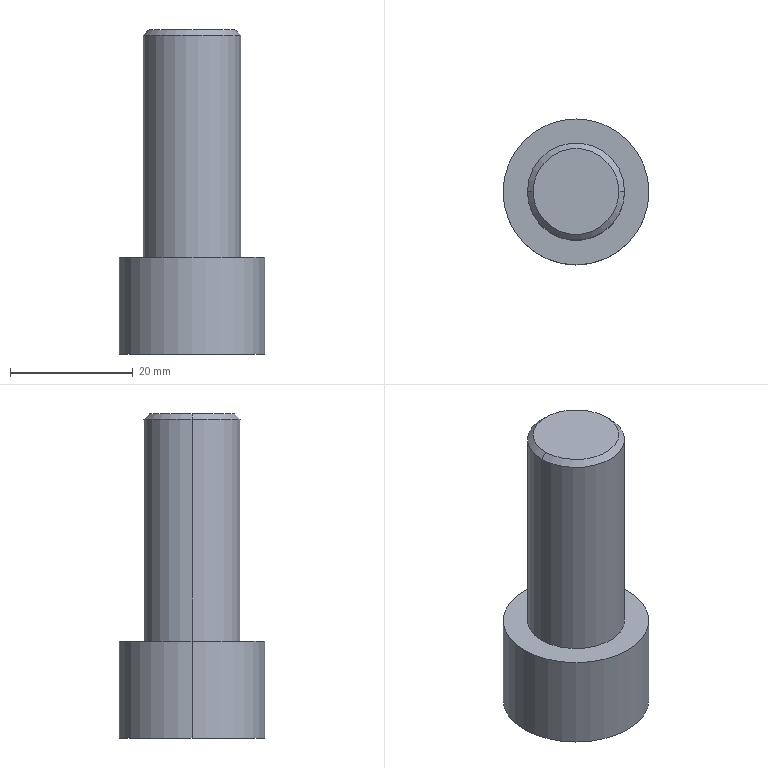Part | STEP file | 4-20.sldasm-Part-232 | 1 solid | 16 faces | box 23.812 x 23.812 x 53.025 mm | volume 12939 mm3 | plane 10 | cylinder 4 | cone 2 | commonest cylinder face diameters 15.875 x2 23.812 x2
STEP:
#1=CARTESIAN_POINT('',(7.,-522.,-80.451));
#2=VERTEX_POINT('',#1);
#3=CARTESIAN_POINT('',(-7.,-522.,-80.451));
#4=VERTEX_POINT('',#3);
#5=CARTESIAN_POINT('',(0.,-522.,-80.451));
#6=DIRECTION('',(0.,0.,1.));
#7=DIRECTION('',(-1.,0.,0.));
#8=AXIS2_PLACEMENT_3D('',#5,#6,#7);
#9=CIRCLE('',#8,7.);
#10=EDGE_CURVE('',#2,#4,#9,.T.);
#11=ORIENTED_EDGE('',*,*,#10,.F.);
#12=CARTESIAN_POINT('',(7.938,-522.,-81.388));
#13=VERTEX_POINT('',#12);
#14=CARTESIAN_POINT('',(7.938,-522.,-81.388));
#15=DIRECTION('',(0.7071,0.,-0.7071));
#16=VECTOR('',#15,1000.);
#17=LINE('',#14,#16);
#18=EDGE_CURVE('',#2,#13,#17,.T.);
#19=ORIENTED_EDGE('',*,*,#18,.T.);
#20=CARTESIAN_POINT('',(-7.938,-522.,-81.388));
#21=VERTEX_POINT('',#20);
#22=CARTESIAN_POINT('',(0.,-522.,-81.388));
#23=DIRECTION('',(0.,0.,-1.));
#24=DIRECTION('',(-1.,0.,0.));
#25=AXIS2_PLACEMENT_3D('',#22,#23,#24);
#26=CIRCLE('',#25,7.938);
#27=EDGE_CURVE('',#21,#13,#26,.T.);
#28=ORIENTED_EDGE('',*,*,#27,.F.);
#29=CARTESIAN_POINT('',(-7.938,-522.,-81.388));
#30=DIRECTION('',(-0.7071,0.,-0.7071));
#31=VECTOR('',#30,1000.);
#32=LINE('',#29,#31);
#33=EDGE_CURVE('',#4,#21,#32,.T.);
#34=ORIENTED_EDGE('',*,*,#33,.F.);
#35=EDGE_LOOP('',(#11,#19,#28,#34));
#36=FACE_OUTER_BOUND('',#35,.T.);
#37=CARTESIAN_POINT('',(0.,-522.,-81.388));
#38=DIRECTION('',(0.,0.,-1.));
#39=DIRECTION('',(-1.,0.,0.));
#40=AXIS2_PLACEMENT_3D('',#37,#38,#39);
#41=CONICAL_SURFACE('',#40,7.938,0.7854);
#42=ADVANCED_FACE('',(#36),#41,.T.);
#43=CARTESIAN_POINT('',(-11.906,-522.,-117.601));
#44=VERTEX_POINT('',#43);
#45=CARTESIAN_POINT('',(11.906,-522.,-117.601));
#46=VERTEX_POINT('',#45);
#47=CARTESIAN_POINT('',(0.,-522.,-117.601));
#48=DIRECTION('',(0.,0.,-1.));
#49=DIRECTION('',(-1.,0.,0.));
#50=AXIS2_PLACEMENT_3D('',#47,#48,#49);
#51=CIRCLE('',#50,11.906);
#52=EDGE_CURVE('',#44,#46,#51,.T.);
#53=ORIENTED_EDGE('',*,*,#52,.T.);
#54=CARTESIAN_POINT('',(11.906,-522.,-133.476));
#55=VERTEX_POINT('',#54);
#56=CARTESIAN_POINT('',(11.906,-522.,-117.601));
#57=DIRECTION('',(0.,0.,-1.));
#58=VECTOR('',#57,1000.);
#59=LINE('',#56,#58);
#60=EDGE_CURVE('',#46,#55,#59,.T.);
#61=ORIENTED_EDGE('',*,*,#60,.T.);
#62=CARTESIAN_POINT('',(-11.906,-522.,-133.476));
#63=VERTEX_POINT('',#62);
#64=CARTESIAN_POINT('',(0.,-522.,-133.476));
#65=DIRECTION('',(0.,0.,-1.));
#66=DIRECTION('',(-1.,0.,0.));
#67=AXIS2_PLACEMENT_3D('',#64,#65,#66);
#68=CIRCLE('',#67,11.906);
#69=EDGE_CURVE('',#63,#55,#68,.T.);
#70=ORIENTED_EDGE('',*,*,#69,.F.);
#71=CARTESIAN_POINT('',(-11.906,-522.,-117.601));
#72=DIRECTION('',(0.,0.,-1.));
#73=VECTOR('',#72,1000.);
#74=LINE('',#71,#73);
#75=EDGE_CURVE('',#44,#63,#74,.T.);
#76=ORIENTED_EDGE('',*,*,#75,.F.);
#77=EDGE_LOOP('',(#53,#61,#70,#76));
#78=FACE_OUTER_BOUND('',#77,.T.);
#79=CARTESIAN_POINT('',(0.,-522.,-117.601));
#80=DIRECTION('',(0.,0.,-1.));
#81=DIRECTION('',(-1.,0.,0.));
#82=AXIS2_PLACEMENT_3D('',#79,#80,#81);
#83=CYLINDRICAL_SURFACE('',#82,11.906);
#84=ADVANCED_FACE('',(#78),#83,.T.);
#85=CARTESIAN_POINT('',(-7.938,-522.,-117.601));
#86=VERTEX_POINT('',#85);
#87=CARTESIAN_POINT('',(7.938,-522.,-117.601));
#88=VERTEX_POINT('',#87);
#89=CARTESIAN_POINT('',(0.,-522.,-117.601));
#90=DIRECTION('',(0.,0.,-1.));
#91=DIRECTION('',(-1.,0.,0.));
#92=AXIS2_PLACEMENT_3D('',#89,#90,#91);
#93=CIRCLE('',#92,7.938);
#94=EDGE_CURVE('',#86,#88,#93,.T.);
#95=ORIENTED_EDGE('',*,*,#94,.F.);
#96=CARTESIAN_POINT('',(-7.938,-522.,-117.601));
#97=DIRECTION('',(0.,0.,1.));
#98=VECTOR('',#97,1000.);
#99=LINE('',#96,#98);
#100=EDGE_CURVE('',#86,#21,#99,.T.);
#101=ORIENTED_EDGE('',*,*,#100,.T.);
#102=ORIENTED_EDGE('',*,*,#27,.T.);
#103=CARTESIAN_POINT('',(7.938,-522.,-117.601));
#104=DIRECTION('',(0.,0.,1.));
#105=VECTOR('',#104,1000.);
#106=LINE('',#103,#105);
#107=EDGE_CURVE('',#88,#13,#106,.T.);
#108=ORIENTED_EDGE('',*,*,#107,.F.);
#109=EDGE_LOOP('',(#95,#101,#102,#108));
#110=FACE_OUTER_BOUND('',#109,.T.);
#111=CARTESIAN_POINT('',(0.,-522.,-117.601));
#112=DIRECTION('',(0.,0.,1.));
#113=DIRECTION('',(1.,0.,0.));
#114=AXIS2_PLACEMENT_3D('',#111,#112,#113);
#115=CYLINDRICAL_SURFACE('',#114,7.938);
#116=ADVANCED_FACE('',(#110),#115,.T.);
#117=ORIENTED_EDGE('',*,*,#100,.F.);
#118=CARTESIAN_POINT('',(0.,-522.,-117.601));
#119=DIRECTION('',(0.,0.,-1.));
#120=DIRECTION('',(-1.,0.,0.));
#121=AXIS2_PLACEMENT_3D('',#118,#119,#120);
#122=CIRCLE('',#121,7.938);
#123=EDGE_CURVE('',#88,#86,#122,.T.);
#124=ORIENTED_EDGE('',*,*,#123,.F.);
#125=ORIENTED_EDGE('',*,*,#107,.T.);
#126=CARTESIAN_POINT('',(0.,-522.,-81.388));
#127=DIRECTION('',(0.,0.,-1.));
#128=DIRECTION('',(-1.,0.,0.));
#129=AXIS2_PLACEMENT_3D('',#126,#127,#128);
#130=CIRCLE('',#129,7.938);
#131=EDGE_CURVE('',#13,#21,#130,.T.);
#132=ORIENTED_EDGE('',*,*,#131,.T.);
#133=EDGE_LOOP('',(#117,#124,#125,#132));
#134=FACE_OUTER_BOUND('',#133,.T.);
#135=CARTESIAN_POINT('',(0.,-522.,-117.601));
#136=DIRECTION('',(0.,0.,1.));
#137=DIRECTION('',(1.,0.,0.));
#138=AXIS2_PLACEMENT_3D('',#135,#136,#137);
#139=CYLINDRICAL_SURFACE('',#138,7.938);
#140=ADVANCED_FACE('',(#134),#139,.T.);
#141=CARTESIAN_POINT('',(0.,-522.,-80.451));
#142=DIRECTION('',(0.,0.,1.));
#143=DIRECTION('',(-1.,0.,0.));
#144=AXIS2_PLACEMENT_3D('',#141,#142,#143);
#145=CIRCLE('',#144,7.);
#146=EDGE_CURVE('',#4,#2,#145,.T.);
#147=ORIENTED_EDGE('',*,*,#146,.T.);
#148=ORIENTED_EDGE('',*,*,#10,.T.);
#149=EDGE_LOOP('',(#147,#148));
#150=FACE_OUTER_BOUND('',#149,.T.);
#151=CARTESIAN_POINT('',(0.,-522.,-80.451));
#152=DIRECTION('',(0.,0.,-1.));
#153=DIRECTION('',(-1.,0.,0.));
#154=AXIS2_PLACEMENT_3D('',#151,#152,#153);
#155=PLANE('',#154);
#156=ADVANCED_FACE('',(#150),#155,.F.);
#157=ORIENTED_EDGE('',*,*,#52,.F.);
#158=CARTESIAN_POINT('',(0.,-522.,-117.601));
#159=DIRECTION('',(0.,0.,-1.));
#160=DIRECTION('',(-1.,0.,0.));
#161=AXIS2_PLACEMENT_3D('',#158,#159,#160);
#162=CIRCLE('',#161,11.906);
#163=EDGE_CURVE('',#46,#44,#162,.T.);
#164=ORIENTED_EDGE('',*,*,#163,.F.);
#165=EDGE_LOOP('',(#157,#164));
#166=FACE_OUTER_BOUND('',#165,.T.);
#167=ORIENTED_EDGE('',*,*,#123,.T.);
#168=ORIENTED_EDGE('',*,*,#94,.T.);
#169=EDGE_LOOP('',(#167,#168));
#170=FACE_BOUND('',#169,.T.);
#171=CARTESIAN_POINT('',(0.,-522.,-117.601));
#172=DIRECTION('',(0.,0.,1.));
#173=DIRECTION('',(1.,0.,0.));
#174=AXIS2_PLACEMENT_3D('',#171,#172,#173);
#175=PLANE('',#174);
#176=ADVANCED_FACE('',(#166,#170),#175,.T.);
#177=CARTESIAN_POINT('',(3.666,-528.35,-133.476));
#178=VERTEX_POINT('',#177);
#179=CARTESIAN_POINT('',(-3.666,-528.35,-133.476));
#180=VERTEX_POINT('',#179);
#181=CARTESIAN_POINT('',(3.666,-528.35,-133.476));
#182=DIRECTION('',(-1.,0.,0.));
#183=VECTOR('',#182,1000.);
#184=LINE('',#181,#183);
#185=EDGE_CURVE('',#178,#180,#184,.T.);
#186=ORIENTED_EDGE('',*,*,#185,.F.);
#187=CARTESIAN_POINT('',(7.332,-522.,-133.476));
#188=VERTEX_POINT('',#187);
#189=CARTESIAN_POINT('',(7.332,-522.,-133.476));
#190=DIRECTION('',(-0.5,-0.866,0.));
#191=VECTOR('',#190,1000.);
#192=LINE('',#189,#191);
#193=EDGE_CURVE('',#188,#178,#192,.T.);
#194=ORIENTED_EDGE('',*,*,#193,.F.);
#195=CARTESIAN_POINT('',(3.666,-515.65,-133.476));
#196=VERTEX_POINT('',#195);
#197=CARTESIAN_POINT('',(3.666,-515.65,-133.476));
#198=DIRECTION('',(0.5,-0.866,0.));
#199=VECTOR('',#198,1000.);
#200=LINE('',#197,#199);
#201=EDGE_CURVE('',#196,#188,#200,.T.);
#202=ORIENTED_EDGE('',*,*,#201,.F.);
#203=CARTESIAN_POINT('',(-3.666,-515.65,-133.476));
#204=VERTEX_POINT('',#203);
#205=CARTESIAN_POINT('',(-3.666,-515.65,-133.476));
#206=DIRECTION('',(1.,0.,0.));
#207=VECTOR('',#206,1000.);
#208=LINE('',#205,#207);
#209=EDGE_CURVE('',#204,#196,#208,.T.);
#210=ORIENTED_EDGE('',*,*,#209,.F.);
#211=CARTESIAN_POINT('',(-7.332,-522.,-133.476));
#212=VERTEX_POINT('',#211);
#213=CARTESIAN_POINT('',(-7.332,-522.,-133.476));
#214=DIRECTION('',(0.5,0.866,0.));
#215=VECTOR('',#214,1000.);
#216=LINE('',#213,#215);
#217=EDGE_CURVE('',#212,#204,#216,.T.);
#218=ORIENTED_EDGE('',*,*,#217,.F.);
#219=CARTESIAN_POINT('',(-3.666,-528.35,-133.476));
#220=DIRECTION('',(-0.5,0.866,0.));
#221=VECTOR('',#220,1000.);
#222=LINE('',#219,#221);
#223=EDGE_CURVE('',#180,#212,#222,.T.);
#224=ORIENTED_EDGE('',*,*,#223,.F.);
#225=EDGE_LOOP('',(#186,#194,#202,#210,#218,#224));
#226=FACE_BOUND('',#225,.T.);
#227=ORIENTED_EDGE('',*,*,#69,.T.);
#228=CARTESIAN_POINT('',(0.,-522.,-133.476));
#229=DIRECTION('',(0.,0.,-1.));
#230=DIRECTION('',(-1.,0.,0.));
#231=AXIS2_PLACEMENT_3D('',#228,#229,#230);
#232=CIRCLE('',#231,11.906);
#233=EDGE_CURVE('',#55,#63,#232,.T.);
#234=ORIENTED_EDGE('',*,*,#233,.T.);
#235=EDGE_LOOP('',(#227,#234));
#236=FACE_OUTER_BOUND('',#235,.T.);
#237=CARTESIAN_POINT('',(0.,-522.,-133.476));
#238=DIRECTION('',(0.,0.,-1.));
#239=DIRECTION('',(-1.,0.,0.));
#240=AXIS2_PLACEMENT_3D('',#237,#238,#239);
#241=PLANE('',#240);
#242=ADVANCED_FACE('',(#226,#236),#241,.T.);
#243=ORIENTED_EDGE('',*,*,#60,.F.);
#244=ORIENTED_EDGE('',*,*,#163,.T.);
#245=ORIENTED_EDGE('',*,*,#75,.T.);
#246=ORIENTED_EDGE('',*,*,#233,.F.);
#247=EDGE_LOOP('',(#243,#244,#245,#246));
#248=FACE_OUTER_BOUND('',#247,.T.);
#249=CARTESIAN_POINT('',(0.,-522.,-117.601));
#250=DIRECTION('',(0.,0.,-1.));
#251=DIRECTION('',(-1.,0.,0.));
#252=AXIS2_PLACEMENT_3D('',#249,#250,#251);
#253=CYLINDRICAL_SURFACE('',#252,11.906);
#254=ADVANCED_FACE('',(#248),#253,.T.);
#255=ORIENTED_EDGE('',*,*,#18,.F.);
#256=ORIENTED_EDGE('',*,*,#146,.F.);
#257=ORIENTED_EDGE('',*,*,#33,.T.);
#258=ORIENTED_EDGE('',*,*,#131,.F.);
#259=EDGE_LOOP('',(#255,#256,#257,#258));
#260=FACE_OUTER_BOUND('',#259,.T.);
#261=CARTESIAN_POINT('',(0.,-522.,-81.388));
#262=DIRECTION('',(0.,0.,-1.));
#263=DIRECTION('',(-1.,0.,0.));
#264=AXIS2_PLACEMENT_3D('',#261,#262,#263);
#265=CONICAL_SURFACE('',#264,7.938,0.7854);
#266=ADVANCED_FACE('',(#260),#265,.T.);
#267=ORIENTED_EDGE('',*,*,#185,.T.);
#268=CARTESIAN_POINT('',(-3.666,-528.35,-122.998));
#269=VERTEX_POINT('',#268);
#270=CARTESIAN_POINT('',(-3.666,-528.35,-122.998));
#271=DIRECTION('',(0.,0.,-1.));
#272=VECTOR('',#271,1000.);
#273=LINE('',#270,#272);
#274=EDGE_CURVE('',#269,#180,#273,.T.);
#275=ORIENTED_EDGE('',*,*,#274,.F.);
#276=CARTESIAN_POINT('',(3.666,-528.35,-122.998));
#277=VERTEX_POINT('',#276);
#278=CARTESIAN_POINT('',(3.666,-528.35,-122.998));
#279=DIRECTION('',(-1.,0.,0.));
#280=VECTOR('',#279,1000.);
#281=LINE('',#278,#280);
#282=EDGE_CURVE('',#277,#269,#281,.T.);
#283=ORIENTED_EDGE('',*,*,#282,.F.);
#284=CARTESIAN_POINT('',(3.666,-528.35,-122.998));
#285=DIRECTION('',(0.,0.,-1.));
#286=VECTOR('',#285,1000.);
#287=LINE('',#284,#286);
#288=EDGE_CURVE('',#277,#178,#287,.T.);
#289=ORIENTED_EDGE('',*,*,#288,.T.);
#290=EDGE_LOOP('',(#267,#275,#283,#289));
#291=FACE_OUTER_BOUND('',#290,.T.);
#292=CARTESIAN_POINT('',(3.666,-528.35,-122.998));
#293=DIRECTION('',(0.,-1.,0.));
#294=DIRECTION('',(0.,0.,1.));
#295=AXIS2_PLACEMENT_3D('',#292,#293,#294);
#296=PLANE('',#295);
#297=ADVANCED_FACE('',(#291),#296,.F.);
#298=ORIENTED_EDGE('',*,*,#223,.T.);
#299=CARTESIAN_POINT('',(-7.332,-522.,-122.998));
#300=VERTEX_POINT('',#299);
#301=CARTESIAN_POINT('',(-7.332,-522.,-122.998));
#302=DIRECTION('',(0.,0.,-1.));
#303=VECTOR('',#302,1000.);
#304=LINE('',#301,#303);
#305=EDGE_CURVE('',#300,#212,#304,.T.);
#306=ORIENTED_EDGE('',*,*,#305,.F.);
#307=CARTESIAN_POINT('',(-3.666,-528.35,-122.998));
#308=DIRECTION('',(-0.5,0.866,0.));
#309=VECTOR('',#308,1000.);
#310=LINE('',#307,#309);
#311=EDGE_CURVE('',#269,#300,#310,.T.);
#312=ORIENTED_EDGE('',*,*,#311,.F.);
#313=ORIENTED_EDGE('',*,*,#274,.T.);
#314=EDGE_LOOP('',(#298,#306,#312,#313));
#315=FACE_OUTER_BOUND('',#314,.T.);
#316=CARTESIAN_POINT('',(-3.666,-528.35,-122.998));
#317=DIRECTION('',(-0.866,-0.5,0.));
#318=DIRECTION('',(-0.5,0.866,0.));
#319=AXIS2_PLACEMENT_3D('',#316,#317,#318);
#320=PLANE('',#319);
#321=ADVANCED_FACE('',(#315),#320,.F.);
#322=ORIENTED_EDGE('',*,*,#217,.T.);
#323=CARTESIAN_POINT('',(-3.666,-515.65,-122.998));
#324=VERTEX_POINT('',#323);
#325=CARTESIAN_POINT('',(-3.666,-515.65,-122.998));
#326=DIRECTION('',(0.,0.,-1.));
#327=VECTOR('',#326,1000.);
#328=LINE('',#325,#327);
#329=EDGE_CURVE('',#324,#204,#328,.T.);
#330=ORIENTED_EDGE('',*,*,#329,.F.);
#331=CARTESIAN_POINT('',(-7.332,-522.,-122.998));
#332=DIRECTION('',(0.5,0.866,0.));
#333=VECTOR('',#332,1000.);
#334=LINE('',#331,#333);
#335=EDGE_CURVE('',#300,#324,#334,.T.);
#336=ORIENTED_EDGE('',*,*,#335,.F.);
#337=ORIENTED_EDGE('',*,*,#305,.T.);
#338=EDGE_LOOP('',(#322,#330,#336,#337));
#339=FACE_OUTER_BOUND('',#338,.T.);
#340=CARTESIAN_POINT('',(-7.332,-522.,-122.998));
#341=DIRECTION('',(-0.866,0.5,0.));
#342=DIRECTION('',(0.5,0.866,0.));
#343=AXIS2_PLACEMENT_3D('',#340,#341,#342);
#344=PLANE('',#343);
#345=ADVANCED_FACE('',(#339),#344,.F.);
#346=ORIENTED_EDGE('',*,*,#209,.T.);
#347=CARTESIAN_POINT('',(3.666,-515.65,-122.998));
#348=VERTEX_POINT('',#347);
#349=CARTESIAN_POINT('',(3.666,-515.65,-122.998));
#350=DIRECTION('',(0.,0.,-1.));
#351=VECTOR('',#350,1000.);
#352=LINE('',#349,#351);
#353=EDGE_CURVE('',#348,#196,#352,.T.);
#354=ORIENTED_EDGE('',*,*,#353,.F.);
#355=CARTESIAN_POINT('',(-3.666,-515.65,-122.998));
#356=DIRECTION('',(1.,0.,0.));
#357=VECTOR('',#356,1000.);
#358=LINE('',#355,#357);
#359=EDGE_CURVE('',#324,#348,#358,.T.);
#360=ORIENTED_EDGE('',*,*,#359,.F.);
#361=ORIENTED_EDGE('',*,*,#329,.T.);
#362=EDGE_LOOP('',(#346,#354,#360,#361));
#363=FACE_OUTER_BOUND('',#362,.T.);
#364=CARTESIAN_POINT('',(-3.666,-515.65,-122.998));
#365=DIRECTION('',(0.,1.,0.));
#366=DIRECTION('',(0.,0.,-1.));
#367=AXIS2_PLACEMENT_3D('',#364,#365,#366);
#368=PLANE('',#367);
#369=ADVANCED_FACE('',(#363),#368,.F.);
#370=ORIENTED_EDGE('',*,*,#201,.T.);
#371=CARTESIAN_POINT('',(7.332,-522.,-122.998));
#372=VERTEX_POINT('',#371);
#373=CARTESIAN_POINT('',(7.332,-522.,-122.998));
#374=DIRECTION('',(0.,0.,-1.));
#375=VECTOR('',#374,1000.);
#376=LINE('',#373,#375);
#377=EDGE_CURVE('',#372,#188,#376,.T.);
#378=ORIENTED_EDGE('',*,*,#377,.F.);
#379=CARTESIAN_POINT('',(3.666,-515.65,-122.998));
#380=DIRECTION('',(0.5,-0.866,0.));
#381=VECTOR('',#380,1000.);
#382=LINE('',#379,#381);
#383=EDGE_CURVE('',#348,#372,#382,.T.);
#384=ORIENTED_EDGE('',*,*,#383,.F.);
#385=ORIENTED_EDGE('',*,*,#353,.T.);
#386=EDGE_LOOP('',(#370,#378,#384,#385));
#387=FACE_OUTER_BOUND('',#386,.T.);
#388=CARTESIAN_POINT('',(3.666,-515.65,-122.998));
#389=DIRECTION('',(0.866,0.5,0.));
#390=DIRECTION('',(0.5,-0.866,0.));
#391=AXIS2_PLACEMENT_3D('',#388,#389,#390);
#392=PLANE('',#391);
#393=ADVANCED_FACE('',(#387),#392,.F.);
#394=ORIENTED_EDGE('',*,*,#193,.T.);
#395=ORIENTED_EDGE('',*,*,#288,.F.);
#396=CARTESIAN_POINT('',(7.332,-522.,-122.998));
#397=DIRECTION('',(-0.5,-0.866,0.));
#398=VECTOR('',#397,1000.);
#399=LINE('',#396,#398);
#400=EDGE_CURVE('',#372,#277,#399,.T.);
#401=ORIENTED_EDGE('',*,*,#400,.F.);
#402=ORIENTED_EDGE('',*,*,#377,.T.);
#403=EDGE_LOOP('',(#394,#395,#401,#402));
#404=FACE_OUTER_BOUND('',#403,.T.);
#405=CARTESIAN_POINT('',(7.332,-522.,-122.998));
#406=DIRECTION('',(0.866,-0.5,0.));
#407=DIRECTION('',(-0.5,-0.866,0.));
#408=AXIS2_PLACEMENT_3D('',#405,#406,#407);
#409=PLANE('',#408);
#410=ADVANCED_FACE('',(#404),#409,.F.);
#411=ORIENTED_EDGE('',*,*,#282,.T.);
#412=ORIENTED_EDGE('',*,*,#311,.T.);
#413=ORIENTED_EDGE('',*,*,#335,.T.);
#414=ORIENTED_EDGE('',*,*,#359,.T.);
#415=ORIENTED_EDGE('',*,*,#383,.T.);
#416=ORIENTED_EDGE('',*,*,#400,.T.);
#417=EDGE_LOOP('',(#411,#412,#413,#414,#415,#416));
#418=FACE_OUTER_BOUND('',#417,.T.);
#419=CARTESIAN_POINT('',(-3.666,-528.35,-122.998));
#420=DIRECTION('',(0.,0.,-1.));
#421=DIRECTION('',(-1.,0.,0.));
#422=AXIS2_PLACEMENT_3D('',#419,#420,#421);
#423=PLANE('',#422);
#424=ADVANCED_FACE('',(#418),#423,.T.);
#425=CLOSED_SHELL('',(#42,#84,#116,#140,#156,#176,#242,#254,#266,#297,#321,#345,#369,#393,#410,#424));
#426=MANIFOLD_SOLID_BREP('',#425);
#427=CARTESIAN_POINT('',(0.,0.,0.));
#428=DIRECTION('',(0.,0.,1.));
#429=DIRECTION('',(1.,0.,0.));
#430=AXIS2_PLACEMENT_3D('',#427,#428,#429);
#431=(LENGTH_UNIT()NAMED_UNIT(*)SI_UNIT(.MILLI.,.METRE.));
#432=UNCERTAINTY_MEASURE_WITH_UNIT(LENGTH_MEASURE(0.00001),#431,'','');
#433=(NAMED_UNIT(*)PLANE_ANGLE_UNIT()SI_UNIT($,.RADIAN.));
#434=(NAMED_UNIT(*)SI_UNIT($,.STERADIAN.)SOLID_ANGLE_UNIT());
#435=(GEOMETRIC_REPRESENTATION_CONTEXT(3)GLOBAL_UNCERTAINTY_ASSIGNED_CONTEXT((#432))GLOBAL_UNIT_ASSIGNED_CONTEXT((#431,#433,#434))REPRESENTATION_CONTEXT('',''));
#436=ADVANCED_BREP_SHAPE_REPRESENTATION('',(#426,#430),#435);